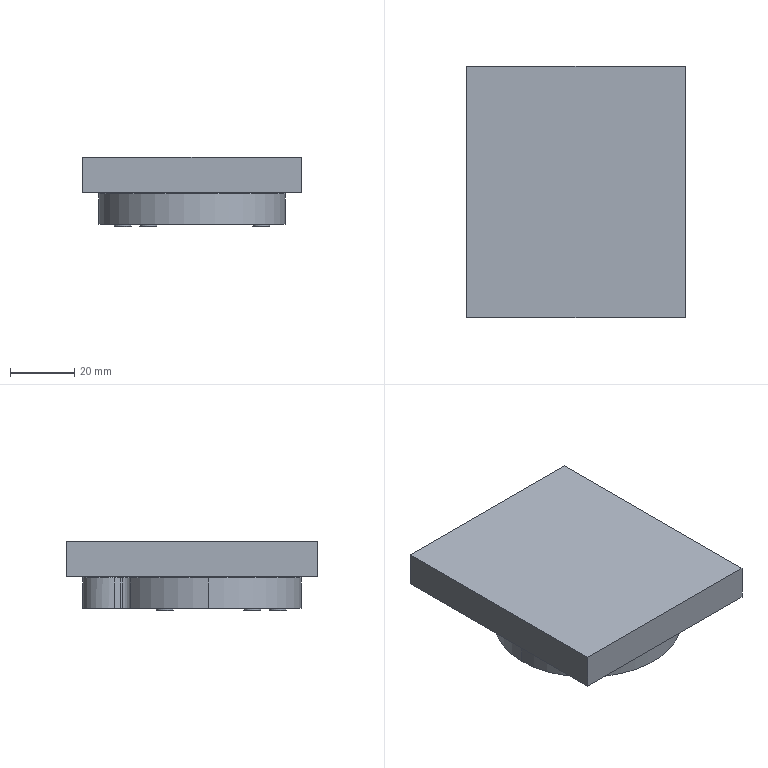NC program | NX | posted with a generic post | part box 68 x 78.27 x 21.8 mm
Lines 1 to 904 of 2405:
N10 G17 G21 G94 G90
(FLOOR_WALL_3 , TOOL : D4)
N12 T11 M6
N14 G54
N16 G17 G0 G90 X0.986 Y-4.966 S9500 M3
N18 G43 Z30. H11
N20 Z1.
N22 G94 G1 X0.957 Y-4.754 Z0.989 F1000.
N24 X0.755 Y-4.435 Z0.969
N26 X0.236 Y-4.091 Z0.936
N28 X-0.137 Y-4.144 Z0.917
N30 X-0.381 Y-4.178 Z0.904
N32 X-0.821 Y-4.513 Z0.875
N34 X-1.024 Y-5.027 Z0.846
N36 X-0.991 Y-5.271 Z0.833
N38 X-0.957 Y-5.516 Z0.82
N40 X-0.622 Y-5.956 Z0.791
N42 X-0.108 Y-6.159 Z0.762
N44 X0.137 Y-6.125 Z0.749
N46 X0.381 Y-6.092 Z0.736
N48 X0.821 Y-5.757 Z0.707
N50 X1.024 Y-5.243 Z0.678
N52 X0.991 Y-4.998 Z0.665
N54 X0.957 Y-4.754 Z0.652
N56 X0.755 Y-4.435 Z0.632
N58 X0.236 Y-4.091 Z0.6
N60 X-0.137 Y-4.144 Z0.58
N62 X-0.381 Y-4.178 Z0.567
N64 X-0.821 Y-4.513 Z0.538
N66 X-1.024 Y-5.027 Z0.509
N68 X-0.991 Y-5.271 Z0.496
N70 X-0.957 Y-5.516 Z0.483
N72 X-0.622 Y-5.956 Z0.454
N74 X-0.108 Y-6.159 Z0.425
N76 X0.137 Y-6.125 Z0.412
N78 X0.381 Y-6.092 Z0.399
N80 X0.821 Y-5.757 Z0.371
N82 X1.024 Y-5.243 Z0.342
N84 X0.991 Y-4.998 Z0.329
N86 X0.957 Y-4.754 Z0.316
N88 X0.755 Y-4.435 Z0.296
N90 X0.236 Y-4.091 Z0.263
N92 X-0.137 Y-4.144 Z0.244
N94 X-0.381 Y-4.178 Z0.231
N96 X-0.821 Y-4.513 Z0.202
N98 X-1.024 Y-5.027 Z0.173
N100 X-0.991 Y-5.271 Z0.16
N102 X-0.957 Y-5.516 Z0.147
N104 X-0.622 Y-5.956 Z0.118
N106 X-0.108 Y-6.159 Z0.089
N108 X0.137 Y-6.125 Z0.076
N110 X0.381 Y-6.092 Z0.063
N112 X0.821 Y-5.757 Z0.034
N114 X1.024 Y-5.243 Z0.005
N116 X0.991 Y-4.998 Z-0.008
N118 X0.957 Y-4.754 Z-0.021
N120 X0.755 Y-4.435 Z-0.041
N122 X0.236 Y-4.091 Z-0.073
N124 X-0.137 Y-4.144 Z-0.093
N126 X-0.381 Y-4.178 Z-0.106
N128 X-0.821 Y-4.513 Z-0.135
N130 X-1.024 Y-5.027 Z-0.164
N132 X-0.991 Y-5.271 Z-0.177
N134 X-0.957 Y-5.516 Z-0.19
N136 X-0.622 Y-5.956 Z-0.219
N138 X-0.108 Y-6.159 Z-0.248
N140 X0.137 Y-6.125 Z-0.261
N142 X0.381 Y-6.092 Z-0.274
N144 X0.821 Y-5.757 Z-0.303
N146 X1.024 Y-5.243 Z-0.332
N148 X0.991 Y-4.998 Z-0.344
N150 X0.957 Y-4.754 Z-0.357
N152 X0.755 Y-4.435 Z-0.377
N154 X0.549 Y-4.299 Z-0.39
N156 X0.393 Y-4.195 Z-0.4
N158 X0.236 Y-4.091 F2500.
N160 X-0.137 Y-4.144
N162 G3 X0.549 Y-4.299 R-1.
N164 G1 X0.393 Y-4.195
N166 X1.501 Y-2.531
N168 G2 X0.712 Y-1.986 R29.
N170 X-0.41 Y-2.163 R29.
N172 G3 X1.648 Y-2.628 R-3.
N174 G1 X1.501 Y-2.531
N176 X2.61 Y-0.866
N178 G2 X1.193 Y0.145 R27.
N180 X-0.683 Y-0.182 R27.
N182 G3 X2.746 Y-0.957 R-5.
N184 G1 X2.61 Y-0.866
N186 X3.718 Y0.798
N188 G2 X1.682 Y2.309 R25.
N190 X-0.956 Y1.8 R25.
N192 G3 X3.845 Y0.715 R-7.
N194 G1 X3.718 Y0.798
N196 X4.827 Y2.463
N198 G2 X2.181 Y4.518 R23.
N200 X-1.229 Y3.781 R23.
N202 G3 X4.943 Y2.386 R-9.
N204 G1 X4.827 Y2.463
N206 X5.935 Y4.128
N208 G2 X2.694 Y6.789 R21.
N210 X-1.502 Y5.762 R21.
N212 G3 X6.042 Y4.057 R-11.
N214 G1 X5.935 Y4.128
N216 X7.044 Y5.792
N218 G2 X3.228 Y9.151 R19.
N220 X-1.776 Y7.743 R19.
N222 G3 X7.14 Y5.729 R-13.
N224 G1 X7.044 Y5.792
N226 X8.153 Y7.457
N228 G2 X3.794 Y11.654 R17.
N230 X-2.049 Y9.725 R17.
N232 G3 X8.239 Y7.4 R-15.
N234 G1 X8.153 Y7.457
N236 X9.261 Y9.122
N238 G2 X4.416 Y14.408 R15.
N240 X-2.322 Y11.706 R15.
N242 G3 X9.337 Y9.071 R-17.
N244 G1 X9.261 Y9.122
N246 X10.37 Y10.786
N248 G2 X5.167 Y17.732 R13.
N250 X-2.595 Y13.687 R13.
N252 G3 X10.436 Y10.743 R-19.
N254 G1 X10.37 Y10.786
N256 X11.479 Y12.451
N258 G2 X6.847 Y24.031 R11.
N260 G1 X7.181 Y25.509
N262 X6.583 Y25.132
N264 X6.359 Y24.141
N266 G2 X-2.868 Y15.668 R11.
N268 G3 X20.803 Y-2.267 R-21.
N270 X11.479 Y12.451 R21.
N272 G1 X12.587 Y14.115
N274 G2 X8.797 Y23.59 R9.
N276 G1 X9.204 Y25.389
N278 G3 X7.505 Y28.08 R2.25
N280 G1 X4.815 Y26.381
N282 X4.408 Y24.582
N284 G2 X-3.141 Y17.65 R9.
N286 G3 X22.784 Y-1.993 R-23.
N288 X12.587 Y14.115 R23.
N290 G1 X13.696 Y15.78
N292 G2 X10.748 Y23.149 R7.
N294 G1 X11.155 Y24.948
N296 G3 X6.902 Y30.133 R4.25
N298 G1 X3.22 Y27.809
N300 G3 X2.864 Y26.822 R4.25
N302 G1 X2.457 Y25.022
N304 G2 X-3.415 Y19.631 R7.
N306 G3 X24.766 Y-1.72 R-25.
N308 X13.696 Y15.78 R25.
N310 G1 X14.804 Y17.445
N312 G2 X12.699 Y22.708 R5.
N314 G1 X13.106 Y24.507
N316 G3 X6.252 Y32.089 R6.25
N318 G1 X1.733 Y29.236
N320 G3 X0.913 Y27.262 R6.25
N322 G1 X0.506 Y25.463
N324 G2 X-3.688 Y21.612 R5.
N326 G3 X26.747 Y-1.447 R-27.
N328 X14.804 Y17.445 R27.
N330 G1 Z0.6
N332 G0 Z3.
N334 X0.986 Y-4.966
N336 Z0.6
N338 G1 X0.957 Y-4.754 Z0.589 F1000.
N340 X0.755 Y-4.435 Z0.569
N342 X0.236 Y-4.091 Z0.536
N344 X-0.137 Y-4.144 Z0.517
N346 X-0.381 Y-4.178 Z0.504
N348 X-0.821 Y-4.513 Z0.475
N350 X-1.024 Y-5.027 Z0.446
N352 X-0.991 Y-5.271 Z0.433
N354 X-0.957 Y-5.516 Z0.42
N356 X-0.622 Y-5.956 Z0.391
N358 X-0.108 Y-6.159 Z0.362
N360 X0.137 Y-6.125 Z0.349
N362 X0.381 Y-6.092 Z0.336
N364 X0.821 Y-5.757 Z0.307
N366 X1.024 Y-5.243 Z0.278
N368 X0.991 Y-4.998 Z0.265
N370 X0.957 Y-4.754 Z0.252
N372 X0.755 Y-4.435 Z0.232
N374 X0.236 Y-4.091 Z0.2
N376 X-0.137 Y-4.144 Z0.18
N378 X-0.381 Y-4.178 Z0.167
N380 X-0.821 Y-4.513 Z0.138
N382 X-1.024 Y-5.027 Z0.109
N384 X-0.991 Y-5.271 Z0.096
N386 X-0.957 Y-5.516 Z0.083
N388 X-0.622 Y-5.956 Z0.054
N390 X-0.108 Y-6.159 Z0.025
N392 X0.137 Y-6.125 Z0.012
N394 X0.381 Y-6.092 Z-0.001
N396 X0.821 Y-5.757 Z-0.029
N398 X1.024 Y-5.243 Z-0.058
N400 X0.991 Y-4.998 Z-0.071
N402 X0.957 Y-4.754 Z-0.084
N404 X0.755 Y-4.435 Z-0.104
N406 X0.236 Y-4.091 Z-0.137
N408 X-0.137 Y-4.144 Z-0.156
N410 X-0.381 Y-4.178 Z-0.169
N412 X-0.821 Y-4.513 Z-0.198
N414 X-1.024 Y-5.027 Z-0.227
N416 X-0.991 Y-5.271 Z-0.24
N418 X-0.957 Y-5.516 Z-0.253
N420 X-0.622 Y-5.956 Z-0.282
N422 X-0.108 Y-6.159 Z-0.311
N424 X0.137 Y-6.125 Z-0.324
N426 X0.381 Y-6.092 Z-0.337
N428 X0.821 Y-5.757 Z-0.366
N430 X1.024 Y-5.243 Z-0.395
N432 X0.991 Y-4.998 Z-0.408
N434 X0.957 Y-4.754 Z-0.421
N436 X0.755 Y-4.435 Z-0.441
N438 X0.236 Y-4.091 Z-0.473
N440 X-0.137 Y-4.144 Z-0.493
N442 X-0.381 Y-4.178 Z-0.506
N444 X-0.821 Y-4.513 Z-0.535
N446 X-1.024 Y-5.027 Z-0.564
N448 X-0.991 Y-5.271 Z-0.577
N450 X-0.957 Y-5.516 Z-0.59
N452 X-0.622 Y-5.956 Z-0.619
N454 X-0.108 Y-6.159 Z-0.648
N456 X0.137 Y-6.125 Z-0.661
N458 X0.381 Y-6.092 Z-0.674
N460 X0.821 Y-5.757 Z-0.703
N462 X1.024 Y-5.243 Z-0.732
N464 X0.991 Y-4.998 Z-0.744
N466 X0.957 Y-4.754 Z-0.757
N468 X0.755 Y-4.435 Z-0.777
N470 X0.549 Y-4.299 Z-0.79
N472 X0.393 Y-4.195 Z-0.8
N474 X0.236 Y-4.091 F2500.
N476 X-0.137 Y-4.144
N478 G3 X0.549 Y-4.299 R-1.
N480 G1 X0.393 Y-4.195
N482 X1.501 Y-2.531
N484 G2 X0.712 Y-1.986 R29.
N486 X-0.41 Y-2.163 R29.
N488 G3 X1.648 Y-2.628 R-3.
N490 G1 X1.501 Y-2.531
N492 X2.61 Y-0.866
N494 G2 X1.193 Y0.145 R27.
N496 X-0.683 Y-0.182 R27.
N498 G3 X2.746 Y-0.957 R-5.
N500 G1 X2.61 Y-0.866
N502 X3.718 Y0.798
N504 G2 X1.682 Y2.309 R25.
N506 X-0.956 Y1.8 R25.
N508 G3 X3.845 Y0.715 R-7.
N510 G1 X3.718 Y0.798
N512 X4.827 Y2.463
N514 G2 X2.181 Y4.518 R23.
N516 X-1.229 Y3.781 R23.
N518 G3 X4.943 Y2.386 R-9.
N520 G1 X4.827 Y2.463
N522 X5.935 Y4.128
N524 G2 X2.694 Y6.789 R21.
N526 X-1.502 Y5.762 R21.
N528 G3 X6.042 Y4.057 R-11.
N530 G1 X5.935 Y4.128
N532 X7.044 Y5.792
N534 G2 X3.228 Y9.151 R19.
N536 X-1.776 Y7.743 R19.
N538 G3 X7.14 Y5.729 R-13.
N540 G1 X7.044 Y5.792
N542 X8.153 Y7.457
N544 G2 X3.794 Y11.654 R17.
N546 X-2.049 Y9.725 R17.
N548 G3 X8.239 Y7.4 R-15.
N550 G1 X8.153 Y7.457
N552 X9.261 Y9.122
N554 G2 X4.416 Y14.408 R15.
N556 X-2.322 Y11.706 R15.
N558 G3 X9.337 Y9.071 R-17.
N560 G1 X9.261 Y9.122
N562 X10.37 Y10.786
N564 G2 X5.167 Y17.732 R13.
N566 X-2.595 Y13.687 R13.
N568 G3 X10.436 Y10.743 R-19.
N570 G1 X10.37 Y10.786
N572 X11.479 Y12.451
N574 G2 X6.847 Y24.031 R11.
N576 G1 X7.181 Y25.509
N578 X6.583 Y25.132
N580 X6.359 Y24.141
N582 G2 X-2.868 Y15.668 R11.
N584 G3 X20.803 Y-2.267 R-21.
N586 X11.479 Y12.451 R21.
N588 G1 X12.587 Y14.115
N590 G2 X8.797 Y23.59 R9.
N592 G1 X9.204 Y25.389
N594 G3 X7.505 Y28.08 R2.25
N596 G1 X4.815 Y26.381
N598 X4.408 Y24.582
N600 G2 X-3.141 Y17.65 R9.
N602 G3 X22.784 Y-1.993 R-23.
N604 X12.587 Y14.115 R23.
N606 G1 X13.696 Y15.78
N608 G2 X10.748 Y23.149 R7.
N610 G1 X11.155 Y24.948
N612 G3 X6.902 Y30.133 R4.25
N614 G1 X3.22 Y27.809
N616 G3 X2.864 Y26.822 R4.25
N618 G1 X2.457 Y25.022
N620 G2 X-3.415 Y19.631 R7.
N622 G3 X24.766 Y-1.72 R-25.
N624 X13.696 Y15.78 R25.
N626 G1 X14.804 Y17.445
N628 G2 X12.699 Y22.708 R5.
N630 G1 X13.106 Y24.507
N632 G3 X6.252 Y32.089 R6.25
N634 G1 X1.733 Y29.236
N636 G3 X0.913 Y27.262 R6.25
N638 G1 X0.506 Y25.463
N640 G2 X-3.688 Y21.612 R5.
N642 G3 X26.747 Y-1.447 R-27.
N644 X14.804 Y17.445 R27.
N646 G1 Z0.2
N648 G0 Z2.6
N650 X0.986 Y-4.966
N652 Z0.2
N654 G1 X0.957 Y-4.754 Z0.189 F1000.
N656 X0.755 Y-4.435 Z0.169
N658 X0.236 Y-4.091 Z0.136
N660 X-0.137 Y-4.144 Z0.117
N662 X-0.381 Y-4.178 Z0.104
N664 X-0.821 Y-4.513 Z0.075
N666 X-1.024 Y-5.027 Z0.046
N668 X-0.991 Y-5.271 Z0.033
N670 X-0.957 Y-5.516 Z0.02
N672 X-0.622 Y-5.956 Z-0.009
N674 X-0.108 Y-6.159 Z-0.038
N676 X0.137 Y-6.125 Z-0.051
N678 X0.381 Y-6.092 Z-0.064
N680 X0.821 Y-5.757 Z-0.093
N682 X1.024 Y-5.243 Z-0.122
N684 X0.991 Y-4.998 Z-0.135
N686 X0.957 Y-4.754 Z-0.148
N688 X0.755 Y-4.435 Z-0.168
N690 X0.236 Y-4.091 Z-0.2
N692 X-0.137 Y-4.144 Z-0.22
N694 X-0.381 Y-4.178 Z-0.233
N696 X-0.821 Y-4.513 Z-0.262
N698 X-1.024 Y-5.027 Z-0.291
N700 X-0.991 Y-5.271 Z-0.304
N702 X-0.957 Y-5.516 Z-0.317
N704 X-0.622 Y-5.956 Z-0.346
N706 X-0.108 Y-6.159 Z-0.375
N708 X0.137 Y-6.125 Z-0.388
N710 X0.381 Y-6.092 Z-0.401
N712 X0.821 Y-5.757 Z-0.429
N714 X1.024 Y-5.243 Z-0.458
N716 X0.991 Y-4.998 Z-0.471
N718 X0.957 Y-4.754 Z-0.484
N720 X0.755 Y-4.435 Z-0.504
N722 X0.236 Y-4.091 Z-0.537
N724 X-0.137 Y-4.144 Z-0.556
N726 X-0.381 Y-4.178 Z-0.569
N728 X-0.821 Y-4.513 Z-0.598
N730 X-1.024 Y-5.027 Z-0.627
N732 X-0.991 Y-5.271 Z-0.64
N734 X-0.957 Y-5.516 Z-0.653
N736 X-0.622 Y-5.956 Z-0.682
N738 X-0.108 Y-6.159 Z-0.711
N740 X0.137 Y-6.125 Z-0.724
N742 X0.381 Y-6.092 Z-0.737
N744 X0.821 Y-5.757 Z-0.766
N746 X1.024 Y-5.243 Z-0.795
N748 X0.991 Y-4.998 Z-0.808
N750 X0.957 Y-4.754 Z-0.821
N752 X0.755 Y-4.435 Z-0.841
N754 X0.236 Y-4.091 Z-0.873
N756 X-0.137 Y-4.144 Z-0.893
N758 X-0.381 Y-4.178 Z-0.906
N760 X-0.821 Y-4.513 Z-0.935
N762 X-1.024 Y-5.027 Z-0.964
N764 X-0.991 Y-5.271 Z-0.977
N766 X-0.957 Y-5.516 Z-0.99
N768 X-0.622 Y-5.956 Z-1.019
N770 X-0.108 Y-6.159 Z-1.048
N772 X0.137 Y-6.125 Z-1.061
N774 X0.381 Y-6.092 Z-1.074
N776 X0.821 Y-5.757 Z-1.103
N778 X1.024 Y-5.243 Z-1.132
N780 X0.991 Y-4.998 Z-1.144
N782 X0.957 Y-4.754 Z-1.157
N784 X0.755 Y-4.435 Z-1.177
N786 X0.549 Y-4.299 Z-1.19
N788 X0.393 Y-4.195 Z-1.2
N790 X0.236 Y-4.091 F2500.
N792 X-0.137 Y-4.144
N794 G3 X0.549 Y-4.299 R-1.
N796 G1 X0.393 Y-4.195
N798 X1.501 Y-2.531
N800 G2 X0.712 Y-1.986 R29.
N802 X-0.41 Y-2.163 R29.
N804 G3 X1.648 Y-2.628 R-3.
N806 G1 X1.501 Y-2.531
N808 X2.61 Y-0.866
N810 G2 X1.193 Y0.145 R27.
N812 X-0.683 Y-0.182 R27.
N814 G3 X2.746 Y-0.957 R-5.
N816 G1 X2.61 Y-0.866
N818 X3.718 Y0.798
N820 G2 X1.682 Y2.309 R25.
N822 X-0.956 Y1.8 R25.
N824 G3 X3.845 Y0.715 R-7.
N826 G1 X3.718 Y0.798
N828 X4.827 Y2.463
N830 G2 X2.181 Y4.518 R23.
N832 X-1.229 Y3.781 R23.
N834 G3 X4.943 Y2.386 R-9.
N836 G1 X4.827 Y2.463
N838 X5.935 Y4.128
N840 G2 X2.694 Y6.789 R21.
N842 X-1.502 Y5.762 R21.
N844 G3 X6.042 Y4.057 R-11.
N846 G1 X5.935 Y4.128
N848 X7.044 Y5.792
N850 G2 X3.228 Y9.151 R19.
N852 X-1.776 Y7.743 R19.
N854 G3 X7.14 Y5.729 R-13.
N856 G1 X7.044 Y5.792
N858 X8.153 Y7.457
N860 G2 X3.794 Y11.654 R17.
N862 X-2.049 Y9.725 R17.
N864 G3 X8.239 Y7.4 R-15.
N866 G1 X8.153 Y7.457
N868 X9.261 Y9.122
N870 G2 X4.416 Y14.408 R15.
N872 X-2.322 Y11.706 R15.
N874 G3 X9.337 Y9.071 R-17.
N876 G1 X9.261 Y9.122
N878 X10.37 Y10.786
N880 G2 X5.167 Y17.732 R13.
N882 X-2.595 Y13.687 R13.
N884 G3 X10.436 Y10.743 R-19.
N886 G1 X10.37 Y10.786
N888 X11.479 Y12.451
N890 G2 X6.847 Y24.031 R11.
N892 G1 X7.181 Y25.509
N894 X6.583 Y25.132
N896 X6.359 Y24.141
N898 G2 X-2.868 Y15.668 R11.
N900 G3 X20.803 Y-2.267 R-21.
N902 X11.479 Y12.451 R21.
N904 G1 X12.587 Y14.115
N906 G2 X8.797 Y23.59 R9.
N908 G1 X9.204 Y25.389
N910 G3 X7.505 Y28.08 R2.25
N912 G1 X4.815 Y26.381
N914 X4.408 Y24.582
N916 G2 X-3.141 Y17.65 R9.
N918 G3 X22.784 Y-1.993 R-23.
N920 X12.587 Y14.115 R23.
N922 G1 X13.696 Y15.78
N924 G2 X10.748 Y23.149 R7.
N926 G1 X11.155 Y24.948
N928 G3 X6.902 Y30.133 R4.25
N930 G1 X3.22 Y27.809
N932 G3 X2.864 Y26.822 R4.25
N934 G1 X2.457 Y25.022
N936 G2 X-3.415 Y19.631 R7.
N938 G3 X24.766 Y-1.72 R-25.
N940 X13.696 Y15.78 R25.
N942 G1 X14.804 Y17.445
N944 G2 X12.699 Y22.708 R5.
N946 G1 X13.106 Y24.507
N948 G3 X6.252 Y32.089 R6.25
N950 G1 X1.733 Y29.236
N952 G3 X0.913 Y27.262 R6.25
N954 G1 X0.506 Y25.463
N956 G2 X-3.688 Y21.612 R5.
N958 G3 X26.747 Y-1.447 R-27.
N960 X14.804 Y17.445 R27.
N962 G1 Z-0.2
N964 G0 Z2.2
N966 X0.986 Y-4.966
N968 Z-0.2
N970 G1 X0.957 Y-4.754 Z-0.211 F1000.
N972 X0.755 Y-4.435 Z-0.231
N974 X0.236 Y-4.091 Z-0.264
N976 X-0.137 Y-4.144 Z-0.283
N978 X-0.381 Y-4.178 Z-0.296
N980 X-0.821 Y-4.513 Z-0.325
N982 X-1.024 Y-5.027 Z-0.354
N984 X-0.991 Y-5.271 Z-0.367
N986 X-0.957 Y-5.516 Z-0.38
N988 X-0.622 Y-5.956 Z-0.409
N990 X-0.108 Y-6.159 Z-0.438
N992 X0.137 Y-6.125 Z-0.451
N994 X0.381 Y-6.092 Z-0.464
N996 X0.821 Y-5.757 Z-0.493
N998 X1.024 Y-5.243 Z-0.522
N1000 X0.991 Y-4.998 Z-0.535
N1002 X0.957 Y-4.754 Z-0.548
N1004 X0.755 Y-4.435 Z-0.568
N1006 X0.236 Y-4.091 Z-0.6
N1008 X-0.137 Y-4.144 Z-0.62
N1010 X-0.381 Y-4.178 Z-0.633
N1012 X-0.821 Y-4.513 Z-0.662
N1014 X-1.024 Y-5.027 Z-0.691
N1016 X-0.991 Y-5.271 Z-0.704
N1018 X-0.957 Y-5.516 Z-0.717
N1020 X-0.622 Y-5.956 Z-0.746
N1022 X-0.108 Y-6.159 Z-0.775
N1024 X0.137 Y-6.125 Z-0.788
N1026 X0.381 Y-6.092 Z-0.801
N1028 X0.821 Y-5.757 Z-0.829
N1030 X1.024 Y-5.243 Z-0.858
N1032 X0.991 Y-4.998 Z-0.871
N1034 X0.957 Y-4.754 Z-0.884
N1036 X0.755 Y-4.435 Z-0.904
N1038 X0.236 Y-4.091 Z-0.937
N1040 X-0.137 Y-4.144 Z-0.956
N1042 X-0.381 Y-4.178 Z-0.969
N1044 X-0.821 Y-4.513 Z-0.998
N1046 X-1.024 Y-5.027 Z-1.027
N1048 X-0.991 Y-5.271 Z-1.04
N1050 X-0.957 Y-5.516 Z-1.053
N1052 X-0.622 Y-5.956 Z-1.082
N1054 X-0.108 Y-6.159 Z-1.111
N1056 X0.137 Y-6.125 Z-1.124
N1058 X0.381 Y-6.092 Z-1.137
N1060 X0.821 Y-5.757 Z-1.166
N1062 X1.024 Y-5.243 Z-1.195
N1064 X0.991 Y-4.998 Z-1.208
N1066 X0.957 Y-4.754 Z-1.221
N1068 X0.755 Y-4.435 Z-1.241
N1070 X0.236 Y-4.091 Z-1.273
N1072 X-0.137 Y-4.144 Z-1.293
N1074 X-0.381 Y-4.178 Z-1.306
N1076 X-0.821 Y-4.513 Z-1.335
N1078 X-1.024 Y-5.027 Z-1.364
N1080 X-0.991 Y-5.271 Z-1.377
N1082 X-0.957 Y-5.516 Z-1.39
N1084 X-0.622 Y-5.956 Z-1.419
N1086 X-0.108 Y-6.159 Z-1.448
N1088 X0.137 Y-6.125 Z-1.461
N1090 X0.381 Y-6.092 Z-1.474
N1092 X0.821 Y-5.757 Z-1.503
N1094 X1.024 Y-5.243 Z-1.532
N1096 X0.991 Y-4.998 Z-1.544
N1098 X0.957 Y-4.754 Z-1.557
N1100 X0.755 Y-4.435 Z-1.577
N1102 X0.549 Y-4.299 Z-1.59
N1104 X0.393 Y-4.195 Z-1.6
N1106 X0.236 Y-4.091 F2500.
N1108 X-0.137 Y-4.144
N1110 G3 X0.549 Y-4.299 R-1.
N1112 G1 X0.393 Y-4.195
N1114 X1.501 Y-2.531
N1116 G2 X0.712 Y-1.986 R29.
N1118 X-0.41 Y-2.163 R29.
N1120 G3 X1.648 Y-2.628 R-3.
N1122 G1 X1.501 Y-2.531
N1124 X2.61 Y-0.866
N1126 G2 X1.193 Y0.145 R27.
N1128 X-0.683 Y-0.182 R27.
N1130 G3 X2.746 Y-0.957 R-5.
N1132 G1 X2.61 Y-0.866
N1134 X3.718 Y0.798
N1136 G2 X1.682 Y2.309 R25.
N1138 X-0.956 Y1.8 R25.
N1140 G3 X3.845 Y0.715 R-7.
N1142 G1 X3.718 Y0.798
N1144 X4.827 Y2.463
N1146 G2 X2.181 Y4.518 R23.
N1148 X-1.229 Y3.781 R23.
N1150 G3 X4.943 Y2.386 R-9.
N1152 G1 X4.827 Y2.463
N1154 X5.935 Y4.128
N1156 G2 X2.694 Y6.789 R21.
N1158 X-1.502 Y5.762 R21.
N1160 G3 X6.042 Y4.057 R-11.
N1162 G1 X5.935 Y4.128
N1164 X7.044 Y5.792
N1166 G2 X3.228 Y9.151 R19.
N1168 X-1.776 Y7.743 R19.
N1170 G3 X7.14 Y5.729 R-13.
N1172 G1 X7.044 Y5.792
N1174 X8.153 Y7.457
N1176 G2 X3.794 Y11.654 R17.
N1178 X-2.049 Y9.725 R17.
N1180 G3 X8.239 Y7.4 R-15.
N1182 G1 X8.153 Y7.457
N1184 X9.261 Y9.122
N1186 G2 X4.416 Y14.408 R15.
N1188 X-2.322 Y11.706 R15.
N1190 G3 X9.337 Y9.071 R-17.
N1192 G1 X9.261 Y9.122
N1194 X10.37 Y10.786
N1196 G2 X5.167 Y17.732 R13.
N1198 X-2.595 Y13.687 R13.
N1200 G3 X10.436 Y10.743 R-19.
N1202 G1 X10.37 Y10.786
N1204 X11.479 Y12.451
N1206 G2 X6.847 Y24.031 R11.
N1208 G1 X7.181 Y25.509
N1210 X6.583 Y25.132
N1212 X6.359 Y24.141
N1214 G2 X-2.868 Y15.668 R11.
N1216 G3 X20.803 Y-2.267 R-21.
N1218 X11.479 Y12.451 R21.
N1220 G1 X12.587 Y14.115
N1222 G2 X8.797 Y23.59 R9.
N1224 G1 X9.204 Y25.389
N1226 G3 X7.505 Y28.08 R2.25
N1228 G1 X4.815 Y26.381
N1230 X4.408 Y24.582
N1232 G2 X-3.141 Y17.65 R9.
N1234 G3 X22.784 Y-1.993 R-23.
N1236 X12.587 Y14.115 R23.
N1238 G1 X13.696 Y15.78
N1240 G2 X10.748 Y23.149 R7.
N1242 G1 X11.155 Y24.948
N1244 G3 X6.902 Y30.133 R4.25
N1246 G1 X3.22 Y27.809
N1248 G3 X2.864 Y26.822 R4.25
N1250 G1 X2.457 Y25.022
N1252 G2 X-3.415 Y19.631 R7.
N1254 G3 X24.766 Y-1.72 R-25.
N1256 X13.696 Y15.78 R25.
N1258 G1 X14.804 Y17.445
N1260 G2 X12.699 Y22.708 R5.
N1262 G1 X13.106 Y24.507
N1264 G3 X6.252 Y32.089 R6.25
N1266 G1 X1.733 Y29.236
N1268 G3 X0.913 Y27.262 R6.25
N1270 G1 X0.506 Y25.463
N1272 G2 X-3.688 Y21.612 R5.
N1274 G3 X26.747 Y-1.447 R-27.
N1276 X14.804 Y17.445 R27.
N1278 G1 Z-0.6
N1280 G0 Z1.8
N1282 X0.986 Y-4.966
N1284 Z-0.6
N1286 G1 X0.957 Y-4.754 Z-0.611 F1000.
N1288 X0.755 Y-4.435 Z-0.631
N1290 X0.236 Y-4.091 Z-0.664
N1292 X-0.137 Y-4.144 Z-0.683
N1294 X-0.381 Y-4.178 Z-0.696
N1296 X-0.821 Y-4.513 Z-0.725
N1298 X-1.024 Y-5.027 Z-0.754
N1300 X-0.991 Y-5.271 Z-0.767
N1302 X-0.957 Y-5.516 Z-0.78
N1304 X-0.622 Y-5.956 Z-0.809
N1306 X-0.108 Y-6.159 Z-0.838
N1308 X0.137 Y-6.125 Z-0.851
N1310 X0.381 Y-6.092 Z-0.864
N1312 X0.821 Y-5.757 Z-0.893
N1314 X1.024 Y-5.243 Z-0.922
N1316 X0.991 Y-4.998 Z-0.935
N1318 X0.957 Y-4.754 Z-0.948
N1320 X0.755 Y-4.435 Z-0.968
N1322 X0.236 Y-4.091 Z-1.
N1324 X-0.137 Y-4.144 Z-1.02
N1326 X-0.381 Y-4.178 Z-1.033
N1328 X-0.821 Y-4.513 Z-1.062
N1330 X-1.024 Y-5.027 Z-1.091
N1332 X-0.991 Y-5.271 Z-1.104
N1334 X-0.957 Y-5.516 Z-1.117
N1336 X-0.622 Y-5.956 Z-1.146
N1338 X-0.108 Y-6.159 Z-1.175
N1340 X0.137 Y-6.125 Z-1.188
N1342 X0.381 Y-6.092 Z-1.201
N1344 X0.821 Y-5.757 Z-1.229
N1346 X1.024 Y-5.243 Z-1.258
N1348 X0.991 Y-4.998 Z-1.271
N1350 X0.957 Y-4.754 Z-1.284
N1352 X0.755 Y-4.435 Z-1.304
N1354 X0.236 Y-4.091 Z-1.337
N1356 X-0.137 Y-4.144 Z-1.356
N1358 X-0.381 Y-4.178 Z-1.369
N1360 X-0.821 Y-4.513 Z-1.398
N1362 X-1.024 Y-5.027 Z-1.427
N1364 X-0.991 Y-5.271 Z-1.44
N1366 X-0.957 Y-5.516 Z-1.453
N1368 X-0.622 Y-5.956 Z-1.482
N1370 X-0.108 Y-6.159 Z-1.511
N1372 X0.137 Y-6.125 Z-1.524
N1374 X0.381 Y-6.092 Z-1.537
N1376 X0.821 Y-5.757 Z-1.566
N1378 X1.024 Y-5.243 Z-1.595
N1380 X0.991 Y-4.998 Z-1.608
N1382 X0.957 Y-4.754 Z-1.621
N1384 X0.755 Y-4.435 Z-1.641
N1386 X0.236 Y-4.091 Z-1.673
N1388 X-0.137 Y-4.144 Z-1.693
N1390 X-0.381 Y-4.178 Z-1.706
N1392 X-0.821 Y-4.513 Z-1.735
N1394 X-1.024 Y-5.027 Z-1.764
N1396 X-0.991 Y-5.271 Z-1.777
N1398 X-0.957 Y-5.516 Z-1.79
N1400 X-0.622 Y-5.956 Z-1.819
N1402 X-0.108 Y-6.159 Z-1.848
N1404 X0.137 Y-6.125 Z-1.861
N1406 X0.381 Y-6.092 Z-1.874
N1408 X0.821 Y-5.757 Z-1.903
N1410 X1.024 Y-5.243 Z-1.932
N1412 X0.991 Y-4.998 Z-1.944
N1414 X0.957 Y-4.754 Z-1.957
N1416 X0.755 Y-4.435 Z-1.977
N1418 X0.549 Y-4.299 Z-1.99
N1420 X0.393 Y-4.195 Z-2.
N1422 X0.236 Y-4.091 F2500.
N1424 X-0.137 Y-4.144
N1426 G3 X0.549 Y-4.299 R-1.
N1428 G1 X0.393 Y-4.195
N1430 X1.501 Y-2.531
N1432 G2 X0.712 Y-1.986 R29.
N1434 X-0.41 Y-2.163 R29.
N1436 G3 X1.648 Y-2.628 R-3.
N1438 G1 X1.501 Y-2.531
N1440 X2.61 Y-0.866
N1442 G2 X1.193 Y0.145 R27.
N1444 X-0.683 Y-0.182 R27.
N1446 G3 X2.746 Y-0.957 R-5.
N1448 G1 X2.61 Y-0.866
N1450 X3.718 Y0.798
N1452 G2 X1.682 Y2.309 R25.
N1454 X-0.956 Y1.8 R25.
N1456 G3 X3.845 Y0.715 R-7.
N1458 G1 X3.718 Y0.798
N1460 X4.827 Y2.463
N1462 G2 X2.181 Y4.518 R23.
N1464 X-1.229 Y3.781 R23.
N1466 G3 X4.943 Y2.386 R-9.
N1468 G1 X4.827 Y2.463
N1470 X5.935 Y4.128
N1472 G2 X2.694 Y6.789 R21.
N1474 X-1.502 Y5.762 R21.
N1476 G3 X6.042 Y4.057 R-11.
N1478 G1 X5.935 Y4.128
N1480 X7.044 Y5.792
N1482 G2 X3.228 Y9.151 R19.
N1484 X-1.776 Y7.743 R19.
N1486 G3 X7.14 Y5.729 R-13.
N1488 G1 X7.044 Y5.792
N1490 X8.153 Y7.457
N1492 G2 X3.794 Y11.654 R17.
N1494 X-2.049 Y9.725 R17.
N1496 G3 X8.239 Y7.4 R-15.
N1498 G1 X8.153 Y7.457
N1500 X9.261 Y9.122
N1502 G2 X4.416 Y14.408 R15.
N1504 X-2.322 Y11.706 R15.
N1506 G3 X9.337 Y9.071 R-17.
N1508 G1 X9.261 Y9.122
N1510 X10.37 Y10.786
N1512 G2 X5.167 Y17.732 R13.
N1514 X-2.595 Y13.687 R13.
N1516 G3 X10.436 Y10.743 R-19.
N1518 G1 X10.37 Y10.786
N1520 X11.479 Y12.451
N1522 G2 X6.847 Y24.031 R11.
N1524 G1 X7.181 Y25.509
N1526 X6.583 Y25.132
N1528 X6.359 Y24.141
N1530 G2 X-2.868 Y15.668 R11.
N1532 G3 X20.803 Y-2.267 R-21.
N1534 X11.479 Y12.451 R21.
N1536 G1 X12.587 Y14.115
N1538 G2 X8.797 Y23.59 R9.
N1540 G1 X9.204 Y25.389
N1542 G3 X7.505 Y28.08 R2.25
N1544 G1 X4.815 Y26.381
N1546 X4.408 Y24.582
N1548 G2 X-3.141 Y17.65 R9.
N1550 G3 X22.784 Y-1.993 R-23.
N1552 X12.587 Y14.115 R23.
N1554 G1 X13.696 Y15.78
N1556 G2 X10.748 Y23.149 R7.
N1558 G1 X11.155 Y24.948
N1560 G3 X6.902 Y30.133 R4.25
N1562 G1 X3.22 Y27.809
N1564 G3 X2.864 Y26.822 R4.25
N1566 G1 X2.457 Y25.022
N1568 G2 X-3.415 Y19.631 R7.
N1570 G3 X24.766 Y-1.72 R-25.
N1572 X13.696 Y15.78 R25.
N1574 G1 X14.804 Y17.445
N1576 G2 X12.699 Y22.708 R5.
N1578 G1 X13.106 Y24.507
N1580 G3 X6.252 Y32.089 R6.25
N1582 G1 X1.733 Y29.236
N1584 G3 X0.913 Y27.262 R6.25
N1586 G1 X0.506 Y25.463
N1588 G2 X-3.688 Y21.612 R5.
N1590 G3 X26.747 Y-1.447 R-27.
N1592 X14.804 Y17.445 R27.
N1594 G1 Z-1.
N1596 G0 Z1.4
N1598 X0.986 Y-4.966
N1600 Z-1.
N1602 G1 X0.957 Y-4.754 Z-1.011 F1000.
N1604 X0.755 Y-4.435 Z-1.031
N1606 X0.236 Y-4.091 Z-1.064
N1608 X-0.137 Y-4.144 Z-1.083
N1610 X-0.381 Y-4.178 Z-1.096
N1612 X-0.821 Y-4.513 Z-1.125
N1614 X-1.024 Y-5.027 Z-1.154
N1616 X-0.991 Y-5.271 Z-1.167
N1618 X-0.957 Y-5.516 Z-1.18
N1620 X-0.622 Y-5.956 Z-1.209
N1622 X-0.108 Y-6.159 Z-1.238
N1624 X0.137 Y-6.125 Z-1.251
N1626 X0.381 Y-6.092 Z-1.264
N1628 X0.821 Y-5.757 Z-1.293
N1630 X1.024 Y-5.243 Z-1.322
N1632 X0.991 Y-4.998 Z-1.335
N1634 X0.957 Y-4.754 Z-1.348
N1636 X0.755 Y-4.435 Z-1.368
N1638 X0.236 Y-4.091 Z-1.4
N1640 X-0.137 Y-4.144 Z-1.42
N1642 X-0.381 Y-4.178 Z-1.433
N1644 X-0.821 Y-4.513 Z-1.462
N1646 X-1.024 Y-5.027 Z-1.491
N1648 X-0.991 Y-5.271 Z-1.504
N1650 X-0.957 Y-5.516 Z-1.517
N1652 X-0.622 Y-5.956 Z-1.546
N1654 X-0.108 Y-6.159 Z-1.575
N1656 X0.137 Y-6.125 Z-1.588
N1658 X0.381 Y-6.092 Z-1.601
N1660 X0.821 Y-5.757 Z-1.629
N1662 X1.024 Y-5.243 Z-1.658
N1664 X0.991 Y-4.998 Z-1.671
N1666 X0.957 Y-4.754 Z-1.684
N1668 X0.755 Y-4.435 Z-1.704
N1670 X0.236 Y-4.091 Z-1.737
N1672 X-0.137 Y-4.144 Z-1.756
N1674 X-0.381 Y-4.178 Z-1.769
N1676 X-0.821 Y-4.513 Z-1.798
N1678 X-1.024 Y-5.027 Z-1.827
N1680 X-0.991 Y-5.271 Z-1.84
N1682 X-0.957 Y-5.516 Z-1.853
N1684 X-0.622 Y-5.956 Z-1.882
N1686 X-0.108 Y-6.159 Z-1.911
N1688 X0.137 Y-6.125 Z-1.924
N1690 X0.381 Y-6.092 Z-1.937
N1692 X0.821 Y-5.757 Z-1.966
N1694 X1.024 Y-5.243 Z-1.995
N1696 X0.991 Y-4.998 Z-2.008
N1698 X0.957 Y-4.754 Z-2.021
N1700 X0.755 Y-4.435 Z-2.041
N1702 X0.236 Y-4.091 Z-2.073
N1704 X-0.137 Y-4.144 Z-2.093
N1706 X-0.381 Y-4.178 Z-2.106
N1708 X-0.821 Y-4.513 Z-2.135
N1710 X-1.024 Y-5.027 Z-2.164
N1712 X-0.991 Y-5.271 Z-2.177
N1714 X-0.957 Y-5.516 Z-2.19
N1716 X-0.622 Y-5.956 Z-2.219
N1718 X-0.108 Y-6.159 Z-2.248
N1720 X0.137 Y-6.125 Z-2.261
N1722 X0.381 Y-6.092 Z-2.274
N1724 X0.821 Y-5.757 Z-2.303
N1726 X1.024 Y-5.243 Z-2.332
N1728 X0.991 Y-4.998 Z-2.344
N1730 X0.957 Y-4.754 Z-2.357
N1732 X0.755 Y-4.435 Z-2.377
N1734 X0.549 Y-4.299 Z-2.39
N1736 X0.393 Y-4.195 Z-2.4
N1738 X0.236 Y-4.091 F2500.
N1740 X-0.137 Y-4.144
N1742 G3 X0.549 Y-4.299 R-1.
N1744 G1 X0.393 Y-4.195
N1746 X1.501 Y-2.531
N1748 G2 X0.712 Y-1.986 R29.
N1750 X-0.41 Y-2.163 R29.
N1752 G3 X1.648 Y-2.628 R-3.
N1754 G1 X1.501 Y-2.531
N1756 X2.61 Y-0.866
N1758 G2 X1.193 Y0.145 R27.
N1760 X-0.683 Y-0.182 R27.
N1762 G3 X2.746 Y-0.957 R-5.
N1764 G1 X2.61 Y-0.866
N1766 X3.718 Y0.798
N1768 G2 X1.682 Y2.309 R25.
N1770 X-0.956 Y1.8 R25.
N1772 G3 X3.845 Y0.715 R-7.
N1774 G1 X3.718 Y0.798
N1776 X4.827 Y2.463
N1778 G2 X2.181 Y4.518 R23.
N1780 X-1.229 Y3.781 R23.
N1782 G3 X4.943 Y2.386 R-9.
N1784 G1 X4.827 Y2.463
N1786 X5.935 Y4.128
N1788 G2 X2.694 Y6.789 R21.
N1790 X-1.502 Y5.762 R21.
N1792 G3 X6.042 Y4.057 R-11.
N1794 G1 X5.935 Y4.128
N1796 X7.044 Y5.792
N1798 G2 X3.228 Y9.151 R19.
N1800 X-1.776 Y7.743 R19.
N1802 G3 X7.14 Y5.729 R-13.
N1804 G1 X7.044 Y5.792
N1806 X8.153 Y7.457